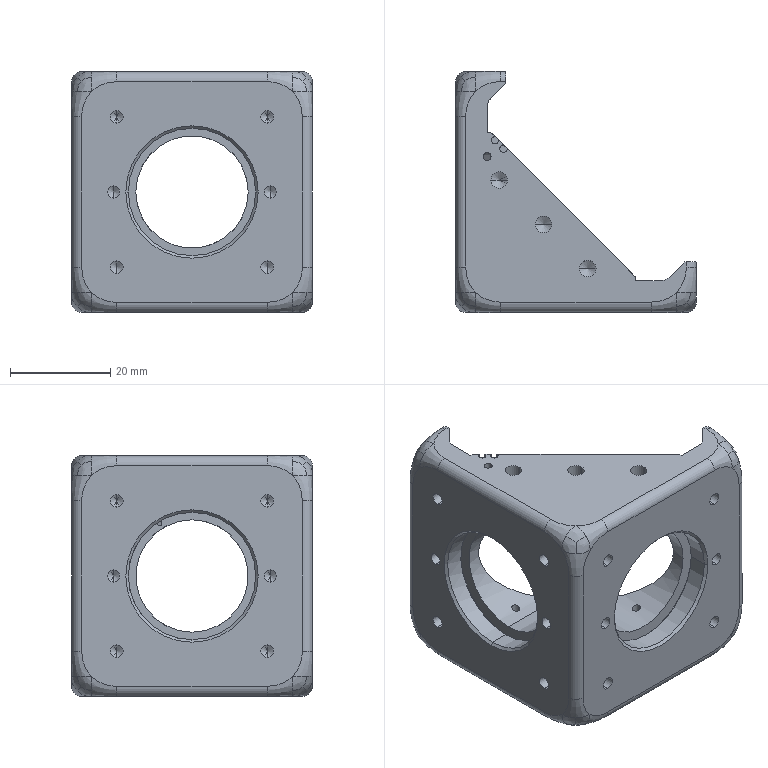Part | STEP file | 1 solid | 435 faces | box 48 x 48 x 48 mm | volume 35050 mm3 | spline 153 | plane 144 | cylinder 98 | cone 40 | commonest cylinder face diameters 4 x21 2.5 x16 1.5 x12 1.6 x12 3.3 x10 2.41 x8